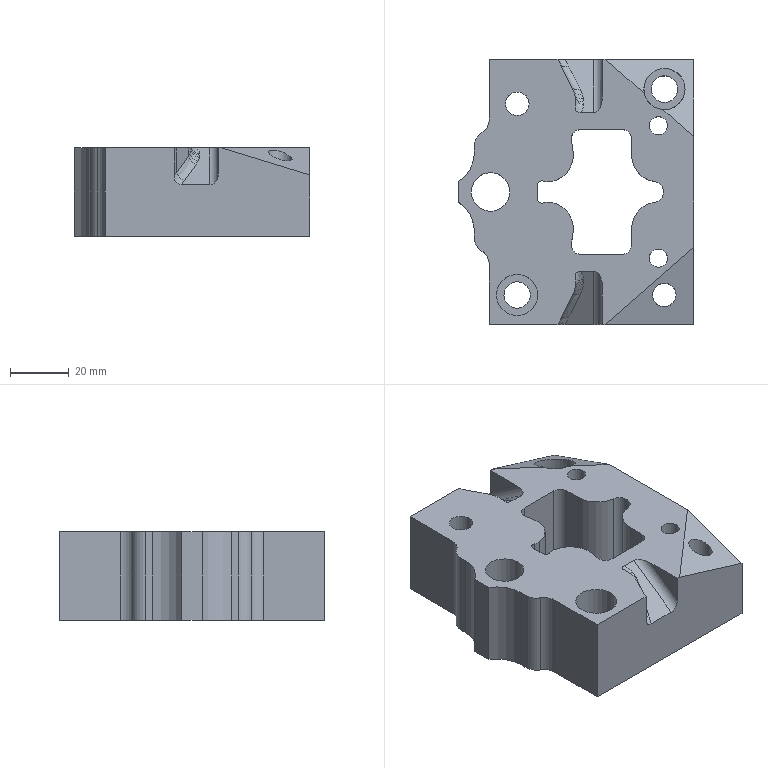Part | STEP file | 1 solid | 85 faces | box 80 x 90 x 30 mm | volume 141495 mm3 | cylinder 34 | plane 26 | spline 25 | commonest cylinder face diameters 6.28 x6 6 x4 10 x4 18.22 x4 3.28 x2 6.2 x2